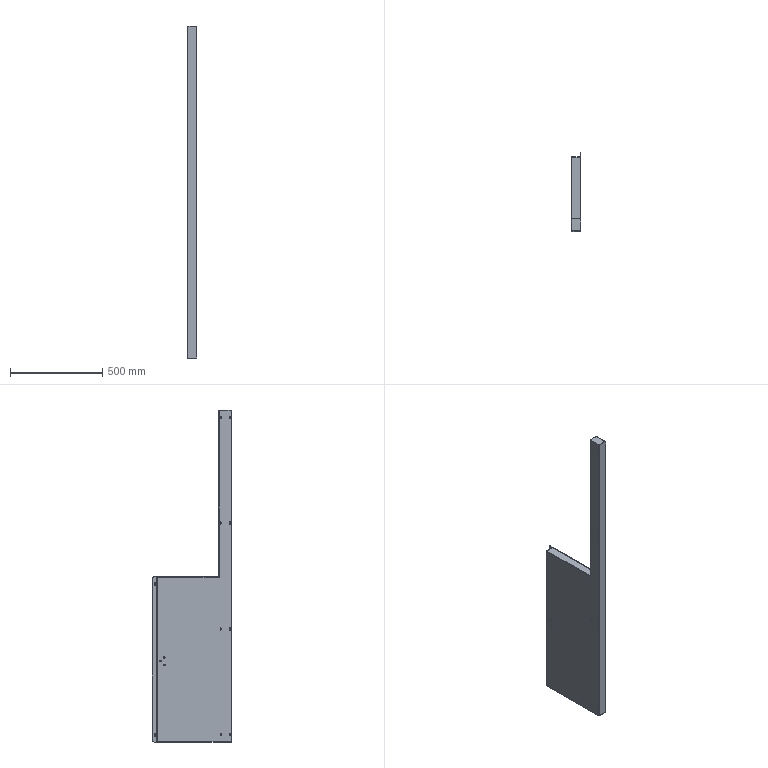Part | SolidWorks | 1 solid | 179 faces | box 50 x 430 x 1800 mm | volume 1098958 mm3 | plane 115 | cylinder 62 | spline 2 | commonest cylinder face diameters 6 x16 2 x12 5 x12 8 x8 7 x6 8.5 x6